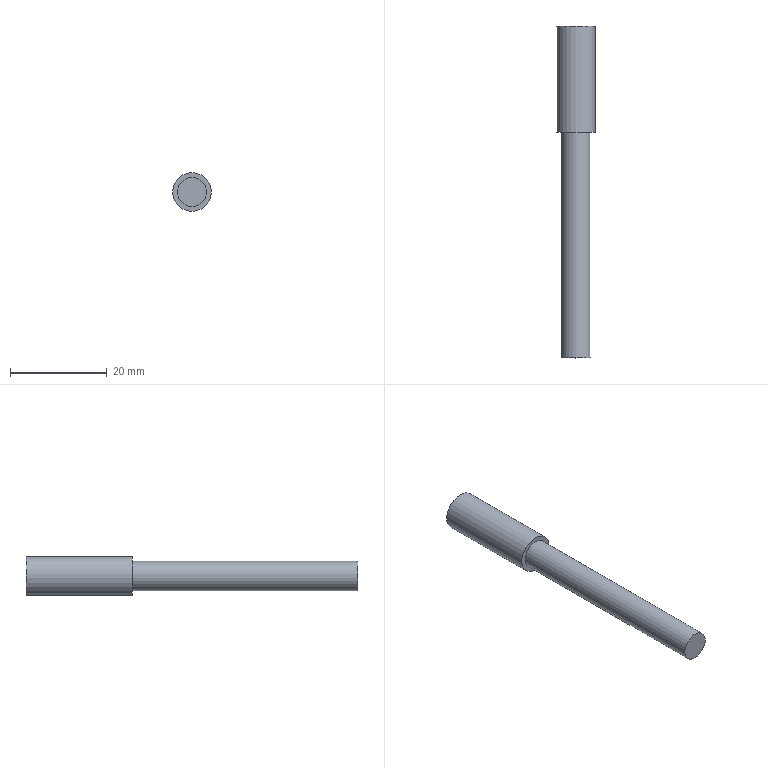Part | NX | features solid 2 | 1 solid | 5 faces | box 8 x 68.5 x 8 mm | volume 2418 mm3 | plane 3 | cylinder 2 | commonest cylinder face diameters 6 x1 8 x1
STEP:
#1=CARTESIAN_POINT('',(-67.,28.5,-32.));
#2=VERTEX_POINT('',#1);
#3=CARTESIAN_POINT('',(-67.,28.5,-35.));
#4=DIRECTION('',(0.,1.,0.));
#5=DIRECTION('',(0.,0.,1.));
#6=AXIS2_PLACEMENT_3D('',#3,#4,#5);
#7=CIRCLE('',#6,3.);
#8=EDGE_CURVE('',#2,#2,#7,.T.);
#9=ORIENTED_EDGE('',*,*,#8,.T.);
#10=EDGE_LOOP('',(#9));
#11=FACE_BOUND('',#10,.T.);
#12=CARTESIAN_POINT('',(-67.,75.1,-38.));
#13=VERTEX_POINT('',#12);
#14=CARTESIAN_POINT('',(-67.,75.1,-35.));
#15=DIRECTION('',(0.,1.,0.));
#16=DIRECTION('',(0.,0.,-1.));
#17=AXIS2_PLACEMENT_3D('',#14,#15,#16);
#18=CIRCLE('',#17,3.);
#19=EDGE_CURVE('',#13,#13,#18,.F.);
#20=ORIENTED_EDGE('',*,*,#19,.T.);
#21=EDGE_LOOP('',(#20));
#22=FACE_BOUND('',#21,.T.);
#23=CARTESIAN_POINT('',(-67.,69.,-35.));
#24=DIRECTION('',(0.,-1.,0.));
#25=DIRECTION('',(-1.,0.,0.));
#26=AXIS2_PLACEMENT_3D('',#23,#24,#25);
#27=CYLINDRICAL_SURFACE('',#26,3.);
#28=ADVANCED_FACE('',(#11,#22),#27,.T.);
#29=ORIENTED_EDGE('',*,*,#8,.F.);
#30=EDGE_LOOP('',(#29));
#31=FACE_BOUND('',#30,.T.);
#32=CARTESIAN_POINT('',(-62.5,28.5,-50.));
#33=DIRECTION('',(0.,-1.,0.));
#34=DIRECTION('',(0.,0.,1.));
#35=AXIS2_PLACEMENT_3D('',#32,#33,#34);
#36=PLANE('',#35);
#37=ADVANCED_FACE('',(#31),#36,.T.);
#38=CARTESIAN_POINT('',(-67.,75.1,-39.));
#39=VERTEX_POINT('',#38);
#40=CARTESIAN_POINT('',(-67.,75.1,-35.));
#41=DIRECTION('',(0.,1.,0.));
#42=DIRECTION('',(0.,0.,-1.));
#43=AXIS2_PLACEMENT_3D('',#40,#41,#42);
#44=CIRCLE('',#43,4.);
#45=EDGE_CURVE('',#39,#39,#44,.T.);
#46=ORIENTED_EDGE('',*,*,#45,.T.);
#47=EDGE_LOOP('',(#46));
#48=FACE_BOUND('',#47,.T.);
#49=CARTESIAN_POINT('',(-67.,97.,-39.));
#50=VERTEX_POINT('',#49);
#51=CARTESIAN_POINT('',(-67.,97.,-35.));
#52=DIRECTION('',(0.,1.,0.));
#53=DIRECTION('',(0.,0.,-1.));
#54=AXIS2_PLACEMENT_3D('',#51,#52,#53);
#55=CIRCLE('',#54,4.);
#56=EDGE_CURVE('',#50,#50,#55,.T.);
#57=ORIENTED_EDGE('',*,*,#56,.F.);
#58=EDGE_LOOP('',(#57));
#59=FACE_BOUND('',#58,.T.);
#60=CARTESIAN_POINT('',(-67.,75.,-35.));
#61=DIRECTION('',(0.,1.,0.));
#62=DIRECTION('',(0.,0.,-1.));
#63=AXIS2_PLACEMENT_3D('',#60,#61,#62);
#64=CYLINDRICAL_SURFACE('',#63,4.);
#65=ADVANCED_FACE('',(#48,#59),#64,.T.);
#66=ORIENTED_EDGE('',*,*,#19,.F.);
#67=EDGE_LOOP('',(#66));
#68=FACE_BOUND('',#67,.T.);
#69=ORIENTED_EDGE('',*,*,#45,.F.);
#70=EDGE_LOOP('',(#69));
#71=FACE_BOUND('',#70,.T.);
#72=CARTESIAN_POINT('',(-67.,75.1,-35.));
#73=DIRECTION('',(0.,1.,0.));
#74=DIRECTION('',(0.,0.,-1.));
#75=AXIS2_PLACEMENT_3D('',#72,#73,#74);
#76=PLANE('',#75);
#77=ADVANCED_FACE('',(#68,#71),#76,.F.);
#78=ORIENTED_EDGE('',*,*,#56,.T.);
#79=EDGE_LOOP('',(#78));
#80=FACE_BOUND('',#79,.T.);
#81=CARTESIAN_POINT('',(-62.5,97.,-50.));
#82=DIRECTION('',(0.,1.,0.));
#83=DIRECTION('',(0.,0.,1.));
#84=AXIS2_PLACEMENT_3D('',#81,#82,#83);
#85=PLANE('',#84);
#86=ADVANCED_FACE('',(#80),#85,.T.);
#87=CLOSED_SHELL('',(#28,#37,#65,#77,#86));
#88=MANIFOLD_SOLID_BREP('',#87);
#89=(LENGTH_UNIT()NAMED_UNIT(*)SI_UNIT(.MILLI.,.METRE.));
#90=UNCERTAINTY_MEASURE_WITH_UNIT(LENGTH_MEASURE(0.00001),#89,'','');
#91=(NAMED_UNIT(*)PLANE_ANGLE_UNIT()SI_UNIT($,.RADIAN.));
#92=(NAMED_UNIT(*)SI_UNIT($,.STERADIAN.)SOLID_ANGLE_UNIT());
#93=(GEOMETRIC_REPRESENTATION_CONTEXT(3)GLOBAL_UNCERTAINTY_ASSIGNED_CONTEXT((#90))GLOBAL_UNIT_ASSIGNED_CONTEXT((#89,#91,#92))REPRESENTATION_CONTEXT('',''));
#94=ADVANCED_BREP_SHAPE_REPRESENTATION('',(#88),#93);